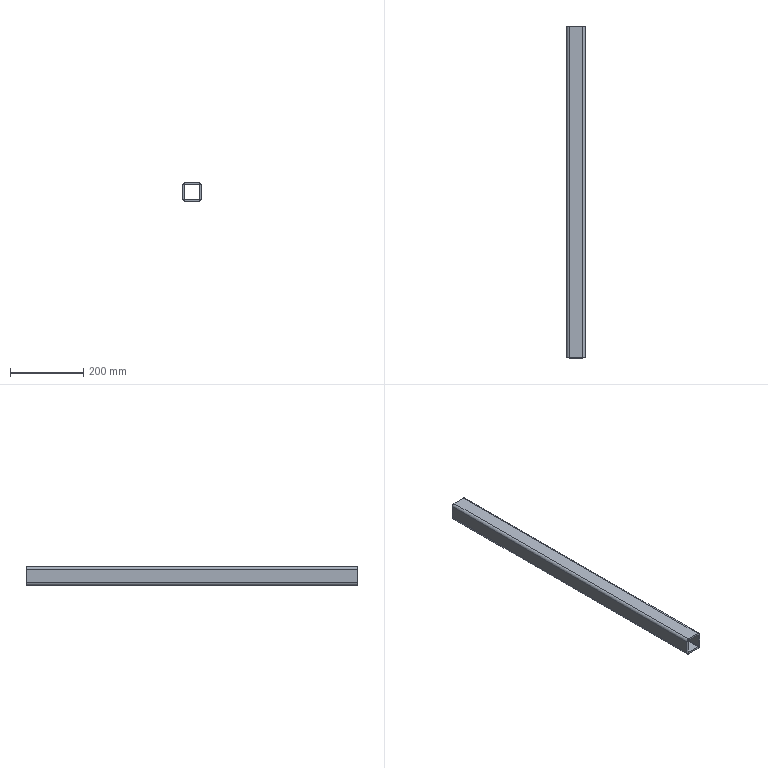Part | NX | 1 solid | 21 faces | box 50 x 906 x 50 mm | volume 780195 mm3 | cylinder 11 | plane 10 | commonest cylinder face diameters 4 x4 14 x4 4.2 x3
STEP:
#1=CARTESIAN_POINT('',(-957.,-25.,600.));
#2=VERTEX_POINT('',#1);
#3=CARTESIAN_POINT('',(-957.,881.,600.));
#4=VERTEX_POINT('',#3);
#5=CARTESIAN_POINT('',(-957.,0.,600.));
#6=DIRECTION('',(0.,1.,0.));
#7=VECTOR('',#6,1000.);
#8=LINE('',#5,#7);
#9=EDGE_CURVE('',#2,#4,#8,.T.);
#10=ORIENTED_EDGE('',*,*,#9,.F.);
#11=CARTESIAN_POINT('',(-950.,-25.,593.));
#12=VERTEX_POINT('',#11);
#13=CARTESIAN_POINT('',(-957.,-25.,593.));
#14=DIRECTION('',(0.,-1.,0.));
#15=DIRECTION('',(1.,0.,0.));
#16=AXIS2_PLACEMENT_3D('',#13,#14,#15);
#17=CIRCLE('',#16,7.);
#18=EDGE_CURVE('',#12,#2,#17,.T.);
#19=ORIENTED_EDGE('',*,*,#18,.F.);
#20=CARTESIAN_POINT('',(-950.,881.,593.));
#21=VERTEX_POINT('',#20);
#22=CARTESIAN_POINT('',(-950.,0.,593.));
#23=DIRECTION('',(0.,1.,0.));
#24=VECTOR('',#23,1000.);
#25=LINE('',#22,#24);
#26=EDGE_CURVE('',#12,#21,#25,.T.);
#27=ORIENTED_EDGE('',*,*,#26,.T.);
#28=CARTESIAN_POINT('',(-957.,881.,593.));
#29=DIRECTION('',(0.,1.,0.));
#30=DIRECTION('',(-1.,0.,0.));
#31=AXIS2_PLACEMENT_3D('',#28,#29,#30);
#32=CIRCLE('',#31,7.);
#33=EDGE_CURVE('',#4,#21,#32,.T.);
#34=ORIENTED_EDGE('',*,*,#33,.F.);
#35=EDGE_LOOP('',(#10,#19,#27,#34));
#36=FACE_BOUND('',#35,.T.);
#37=CARTESIAN_POINT('',(-957.,0.,593.));
#38=DIRECTION('',(0.,1.,0.));
#39=DIRECTION('',(-1.,0.,0.));
#40=AXIS2_PLACEMENT_3D('',#37,#38,#39);
#41=CYLINDRICAL_SURFACE('',#40,7.);
#42=ADVANCED_FACE('',(#36),#41,.T.);
#43=CARTESIAN_POINT('',(-993.,-25.,600.));
#44=VERTEX_POINT('',#43);
#45=CARTESIAN_POINT('',(-993.,881.,600.));
#46=VERTEX_POINT('',#45);
#47=CARTESIAN_POINT('',(-993.,0.,600.));
#48=DIRECTION('',(0.,1.,0.));
#49=VECTOR('',#48,1000.);
#50=LINE('',#47,#49);
#51=EDGE_CURVE('',#44,#46,#50,.T.);
#52=ORIENTED_EDGE('',*,*,#51,.F.);
#53=CARTESIAN_POINT('',(-957.,-25.,600.));
#54=DIRECTION('',(-1.,0.,0.));
#55=VECTOR('',#54,1000.);
#56=LINE('',#53,#55);
#57=EDGE_CURVE('',#2,#44,#56,.T.);
#58=ORIENTED_EDGE('',*,*,#57,.F.);
#59=ORIENTED_EDGE('',*,*,#9,.T.);
#60=CARTESIAN_POINT('',(-957.,881.,600.));
#61=DIRECTION('',(1.,0.,0.));
#62=VECTOR('',#61,1000.);
#63=LINE('',#60,#62);
#64=EDGE_CURVE('',#46,#4,#63,.T.);
#65=ORIENTED_EDGE('',*,*,#64,.F.);
#66=EDGE_LOOP('',(#52,#58,#59,#65));
#67=FACE_BOUND('',#66,.T.);
#68=CARTESIAN_POINT('',(-957.,0.,600.));
#69=DIRECTION('',(0.,0.,-1.));
#70=DIRECTION('',(-1.,0.,0.));
#71=AXIS2_PLACEMENT_3D('',#68,#69,#70);
#72=PLANE('',#71);
#73=ADVANCED_FACE('',(#67),#72,.F.);
#74=CARTESIAN_POINT('',(-1000.,-25.,593.));
#75=VERTEX_POINT('',#74);
#76=CARTESIAN_POINT('',(-1000.,881.,593.));
#77=VERTEX_POINT('',#76);
#78=CARTESIAN_POINT('',(-1000.,0.,593.));
#79=DIRECTION('',(0.,1.,0.));
#80=VECTOR('',#79,1000.);
#81=LINE('',#78,#80);
#82=EDGE_CURVE('',#75,#77,#81,.T.);
#83=ORIENTED_EDGE('',*,*,#82,.F.);
#84=CARTESIAN_POINT('',(-993.,-25.,593.));
#85=DIRECTION('',(0.,-1.,0.));
#86=DIRECTION('',(1.,0.,0.));
#87=AXIS2_PLACEMENT_3D('',#84,#85,#86);
#88=CIRCLE('',#87,7.);
#89=EDGE_CURVE('',#44,#75,#88,.T.);
#90=ORIENTED_EDGE('',*,*,#89,.F.);
#91=ORIENTED_EDGE('',*,*,#51,.T.);
#92=CARTESIAN_POINT('',(-993.,881.,593.));
#93=DIRECTION('',(0.,1.,0.));
#94=DIRECTION('',(-1.,0.,0.));
#95=AXIS2_PLACEMENT_3D('',#92,#93,#94);
#96=CIRCLE('',#95,7.);
#97=EDGE_CURVE('',#77,#46,#96,.T.);
#98=ORIENTED_EDGE('',*,*,#97,.F.);
#99=EDGE_LOOP('',(#83,#90,#91,#98));
#100=FACE_BOUND('',#99,.T.);
#101=CARTESIAN_POINT('',(-993.,0.,593.));
#102=DIRECTION('',(0.,1.,0.));
#103=DIRECTION('',(-1.,0.,0.));
#104=AXIS2_PLACEMENT_3D('',#101,#102,#103);
#105=CYLINDRICAL_SURFACE('',#104,7.);
#106=ADVANCED_FACE('',(#100),#105,.T.);
#107=CARTESIAN_POINT('',(-1000.,-25.,557.));
#108=VERTEX_POINT('',#107);
#109=CARTESIAN_POINT('',(-1000.,881.,557.));
#110=VERTEX_POINT('',#109);
#111=CARTESIAN_POINT('',(-1000.,0.,557.));
#112=DIRECTION('',(0.,1.,0.));
#113=VECTOR('',#112,1000.);
#114=LINE('',#111,#113);
#115=EDGE_CURVE('',#108,#110,#114,.T.);
#116=ORIENTED_EDGE('',*,*,#115,.F.);
#117=CARTESIAN_POINT('',(-1000.,-25.,557.));
#118=DIRECTION('',(0.,0.,-1.));
#119=VECTOR('',#118,1000.);
#120=LINE('',#117,#119);
#121=EDGE_CURVE('',#75,#108,#120,.T.);
#122=ORIENTED_EDGE('',*,*,#121,.F.);
#123=ORIENTED_EDGE('',*,*,#82,.T.);
#124=CARTESIAN_POINT('',(-1000.,881.,557.));
#125=DIRECTION('',(0.,0.,1.));
#126=VECTOR('',#125,1000.);
#127=LINE('',#124,#126);
#128=EDGE_CURVE('',#110,#77,#127,.T.);
#129=ORIENTED_EDGE('',*,*,#128,.F.);
#130=EDGE_LOOP('',(#116,#122,#123,#129));
#131=FACE_BOUND('',#130,.T.);
#132=CARTESIAN_POINT('',(-1000.,0.,557.));
#133=DIRECTION('',(1.,0.,0.));
#134=DIRECTION('',(0.,1.,0.));
#135=AXIS2_PLACEMENT_3D('',#132,#133,#134);
#136=PLANE('',#135);
#137=ADVANCED_FACE('',(#131),#136,.F.);
#138=CARTESIAN_POINT('',(-993.,-25.,550.));
#139=VERTEX_POINT('',#138);
#140=CARTESIAN_POINT('',(-993.,881.,550.));
#141=VERTEX_POINT('',#140);
#142=CARTESIAN_POINT('',(-993.,0.,550.));
#143=DIRECTION('',(0.,1.,0.));
#144=VECTOR('',#143,1000.);
#145=LINE('',#142,#144);
#146=EDGE_CURVE('',#139,#141,#145,.T.);
#147=ORIENTED_EDGE('',*,*,#146,.F.);
#148=CARTESIAN_POINT('',(-993.,-25.,557.));
#149=DIRECTION('',(0.,-1.,0.));
#150=DIRECTION('',(1.,0.,0.));
#151=AXIS2_PLACEMENT_3D('',#148,#149,#150);
#152=CIRCLE('',#151,7.);
#153=EDGE_CURVE('',#108,#139,#152,.T.);
#154=ORIENTED_EDGE('',*,*,#153,.F.);
#155=ORIENTED_EDGE('',*,*,#115,.T.);
#156=CARTESIAN_POINT('',(-993.,881.,557.));
#157=DIRECTION('',(0.,1.,0.));
#158=DIRECTION('',(-1.,0.,0.));
#159=AXIS2_PLACEMENT_3D('',#156,#157,#158);
#160=CIRCLE('',#159,7.);
#161=EDGE_CURVE('',#141,#110,#160,.T.);
#162=ORIENTED_EDGE('',*,*,#161,.F.);
#163=EDGE_LOOP('',(#147,#154,#155,#162));
#164=FACE_BOUND('',#163,.T.);
#165=CARTESIAN_POINT('',(-993.,0.,557.));
#166=DIRECTION('',(0.,1.,0.));
#167=DIRECTION('',(-1.,0.,0.));
#168=AXIS2_PLACEMENT_3D('',#165,#166,#167);
#169=CYLINDRICAL_SURFACE('',#168,7.);
#170=ADVANCED_FACE('',(#164),#169,.T.);
#171=CARTESIAN_POINT('',(-975.,133.1,550.));
#172=VERTEX_POINT('',#171);
#173=CARTESIAN_POINT('',(-975.,131.,550.));
#174=DIRECTION('',(0.,0.,-1.));
#175=DIRECTION('',(0.,1.,0.));
#176=AXIS2_PLACEMENT_3D('',#173,#174,#175);
#177=CIRCLE('',#176,2.1);
#178=EDGE_CURVE('',#172,#172,#177,.T.);
#179=ORIENTED_EDGE('',*,*,#178,.F.);
#180=EDGE_LOOP('',(#179));
#181=FACE_BOUND('',#180,.T.);
#182=CARTESIAN_POINT('',(-975.,433.1,550.));
#183=VERTEX_POINT('',#182);
#184=CARTESIAN_POINT('',(-975.,431.,550.));
#185=DIRECTION('',(0.,0.,-1.));
#186=DIRECTION('',(0.,1.,0.));
#187=AXIS2_PLACEMENT_3D('',#184,#185,#186);
#188=CIRCLE('',#187,2.1);
#189=EDGE_CURVE('',#183,#183,#188,.T.);
#190=ORIENTED_EDGE('',*,*,#189,.F.);
#191=EDGE_LOOP('',(#190));
#192=FACE_BOUND('',#191,.T.);
#193=CARTESIAN_POINT('',(-975.,733.1,550.));
#194=VERTEX_POINT('',#193);
#195=CARTESIAN_POINT('',(-975.,731.,550.));
#196=DIRECTION('',(0.,0.,-1.));
#197=DIRECTION('',(0.,1.,0.));
#198=AXIS2_PLACEMENT_3D('',#195,#196,#197);
#199=CIRCLE('',#198,2.1);
#200=EDGE_CURVE('',#194,#194,#199,.T.);
#201=ORIENTED_EDGE('',*,*,#200,.F.);
#202=EDGE_LOOP('',(#201));
#203=FACE_BOUND('',#202,.T.);
#204=CARTESIAN_POINT('',(-957.,-25.,550.));
#205=VERTEX_POINT('',#204);
#206=CARTESIAN_POINT('',(-957.,881.,550.));
#207=VERTEX_POINT('',#206);
#208=CARTESIAN_POINT('',(-957.,0.,550.));
#209=DIRECTION('',(0.,1.,0.));
#210=VECTOR('',#209,1000.);
#211=LINE('',#208,#210);
#212=EDGE_CURVE('',#205,#207,#211,.T.);
#213=ORIENTED_EDGE('',*,*,#212,.F.);
#214=CARTESIAN_POINT('',(-993.,-25.,550.));
#215=DIRECTION('',(1.,0.,0.));
#216=VECTOR('',#215,1000.);
#217=LINE('',#214,#216);
#218=EDGE_CURVE('',#139,#205,#217,.T.);
#219=ORIENTED_EDGE('',*,*,#218,.F.);
#220=ORIENTED_EDGE('',*,*,#146,.T.);
#221=CARTESIAN_POINT('',(-993.,881.,550.));
#222=DIRECTION('',(-1.,0.,0.));
#223=VECTOR('',#222,1000.);
#224=LINE('',#221,#223);
#225=EDGE_CURVE('',#207,#141,#224,.T.);
#226=ORIENTED_EDGE('',*,*,#225,.F.);
#227=EDGE_LOOP('',(#213,#219,#220,#226));
#228=FACE_BOUND('',#227,.T.);
#229=CARTESIAN_POINT('',(-993.,0.,550.));
#230=DIRECTION('',(0.,0.,1.));
#231=DIRECTION('',(1.,0.,0.));
#232=AXIS2_PLACEMENT_3D('',#229,#230,#231);
#233=PLANE('',#232);
#234=ADVANCED_FACE('',(#181,#192,#203,#228),#233,.F.);
#235=CARTESIAN_POINT('',(-950.,-25.,557.));
#236=VERTEX_POINT('',#235);
#237=CARTESIAN_POINT('',(-950.,881.,557.));
#238=VERTEX_POINT('',#237);
#239=CARTESIAN_POINT('',(-950.,0.,557.));
#240=DIRECTION('',(0.,1.,0.));
#241=VECTOR('',#240,1000.);
#242=LINE('',#239,#241);
#243=EDGE_CURVE('',#236,#238,#242,.T.);
#244=ORIENTED_EDGE('',*,*,#243,.F.);
#245=CARTESIAN_POINT('',(-957.,-25.,557.));
#246=DIRECTION('',(0.,-1.,0.));
#247=DIRECTION('',(1.,0.,0.));
#248=AXIS2_PLACEMENT_3D('',#245,#246,#247);
#249=CIRCLE('',#248,7.);
#250=EDGE_CURVE('',#205,#236,#249,.T.);
#251=ORIENTED_EDGE('',*,*,#250,.F.);
#252=ORIENTED_EDGE('',*,*,#212,.T.);
#253=CARTESIAN_POINT('',(-957.,881.,557.));
#254=DIRECTION('',(0.,1.,0.));
#255=DIRECTION('',(-1.,0.,0.));
#256=AXIS2_PLACEMENT_3D('',#253,#254,#255);
#257=CIRCLE('',#256,7.);
#258=EDGE_CURVE('',#238,#207,#257,.T.);
#259=ORIENTED_EDGE('',*,*,#258,.F.);
#260=EDGE_LOOP('',(#244,#251,#252,#259));
#261=FACE_BOUND('',#260,.T.);
#262=CARTESIAN_POINT('',(-957.,0.,557.));
#263=DIRECTION('',(0.,1.,0.));
#264=DIRECTION('',(-1.,0.,0.));
#265=AXIS2_PLACEMENT_3D('',#262,#263,#264);
#266=CYLINDRICAL_SURFACE('',#265,7.);
#267=ADVANCED_FACE('',(#261),#266,.T.);
#268=CARTESIAN_POINT('',(-993.,-25.,595.));
#269=VERTEX_POINT('',#268);
#270=CARTESIAN_POINT('',(-993.,881.,595.));
#271=VERTEX_POINT('',#270);
#272=CARTESIAN_POINT('',(-993.,0.,595.));
#273=DIRECTION('',(0.,1.,0.));
#274=VECTOR('',#273,1000.);
#275=LINE('',#272,#274);
#276=EDGE_CURVE('',#269,#271,#275,.T.);
#277=ORIENTED_EDGE('',*,*,#276,.F.);
#278=CARTESIAN_POINT('',(-995.,-25.,593.));
#279=VERTEX_POINT('',#278);
#280=CARTESIAN_POINT('',(-993.,-25.,593.));
#281=DIRECTION('',(0.,-1.,0.));
#282=DIRECTION('',(1.,0.,0.));
#283=AXIS2_PLACEMENT_3D('',#280,#281,#282);
#284=CIRCLE('',#283,2.);
#285=EDGE_CURVE('',#269,#279,#284,.T.);
#286=ORIENTED_EDGE('',*,*,#285,.T.);
#287=CARTESIAN_POINT('',(-995.,881.,593.));
#288=VERTEX_POINT('',#287);
#289=CARTESIAN_POINT('',(-995.,0.,593.));
#290=DIRECTION('',(0.,1.,0.));
#291=VECTOR('',#290,1000.);
#292=LINE('',#289,#291);
#293=EDGE_CURVE('',#279,#288,#292,.T.);
#294=ORIENTED_EDGE('',*,*,#293,.T.);
#295=CARTESIAN_POINT('',(-993.,881.,593.));
#296=DIRECTION('',(0.,1.,0.));
#297=DIRECTION('',(-1.,0.,0.));
#298=AXIS2_PLACEMENT_3D('',#295,#296,#297);
#299=CIRCLE('',#298,2.);
#300=EDGE_CURVE('',#288,#271,#299,.T.);
#301=ORIENTED_EDGE('',*,*,#300,.T.);
#302=EDGE_LOOP('',(#277,#286,#294,#301));
#303=FACE_BOUND('',#302,.T.);
#304=CARTESIAN_POINT('',(-993.,0.,593.));
#305=DIRECTION('',(0.,1.,0.));
#306=DIRECTION('',(-1.,0.,0.));
#307=AXIS2_PLACEMENT_3D('',#304,#305,#306);
#308=CYLINDRICAL_SURFACE('',#307,2.);
#309=ADVANCED_FACE('',(#303),#308,.F.);
#310=CARTESIAN_POINT('',(-957.,-25.,595.));
#311=VERTEX_POINT('',#310);
#312=CARTESIAN_POINT('',(-957.,881.,595.));
#313=VERTEX_POINT('',#312);
#314=CARTESIAN_POINT('',(-957.,0.,595.));
#315=DIRECTION('',(0.,1.,0.));
#316=VECTOR('',#315,1000.);
#317=LINE('',#314,#316);
#318=EDGE_CURVE('',#311,#313,#317,.T.);
#319=ORIENTED_EDGE('',*,*,#318,.F.);
#320=CARTESIAN_POINT('',(-957.,-25.,595.));
#321=DIRECTION('',(-1.,0.,0.));
#322=VECTOR('',#321,1000.);
#323=LINE('',#320,#322);
#324=EDGE_CURVE('',#311,#269,#323,.T.);
#325=ORIENTED_EDGE('',*,*,#324,.T.);
#326=ORIENTED_EDGE('',*,*,#276,.T.);
#327=CARTESIAN_POINT('',(-957.,881.,595.));
#328=DIRECTION('',(1.,0.,0.));
#329=VECTOR('',#328,1000.);
#330=LINE('',#327,#329);
#331=EDGE_CURVE('',#271,#313,#330,.T.);
#332=ORIENTED_EDGE('',*,*,#331,.T.);
#333=EDGE_LOOP('',(#319,#325,#326,#332));
#334=FACE_BOUND('',#333,.T.);
#335=CARTESIAN_POINT('',(-957.,0.,595.));
#336=DIRECTION('',(0.,0.,-1.));
#337=DIRECTION('',(-1.,0.,0.));
#338=AXIS2_PLACEMENT_3D('',#335,#336,#337);
#339=PLANE('',#338);
#340=ADVANCED_FACE('',(#334),#339,.T.);
#341=CARTESIAN_POINT('',(-955.,-25.,593.));
#342=VERTEX_POINT('',#341);
#343=CARTESIAN_POINT('',(-955.,881.,593.));
#344=VERTEX_POINT('',#343);
#345=CARTESIAN_POINT('',(-955.,0.,593.));
#346=DIRECTION('',(0.,1.,0.));
#347=VECTOR('',#346,1000.);
#348=LINE('',#345,#347);
#349=EDGE_CURVE('',#342,#344,#348,.T.);
#350=ORIENTED_EDGE('',*,*,#349,.F.);
#351=CARTESIAN_POINT('',(-957.,-25.,593.));
#352=DIRECTION('',(0.,-1.,0.));
#353=DIRECTION('',(1.,0.,0.));
#354=AXIS2_PLACEMENT_3D('',#351,#352,#353);
#355=CIRCLE('',#354,2.);
#356=EDGE_CURVE('',#342,#311,#355,.T.);
#357=ORIENTED_EDGE('',*,*,#356,.T.);
#358=ORIENTED_EDGE('',*,*,#318,.T.);
#359=CARTESIAN_POINT('',(-957.,881.,593.));
#360=DIRECTION('',(0.,1.,0.));
#361=DIRECTION('',(-1.,0.,0.));
#362=AXIS2_PLACEMENT_3D('',#359,#360,#361);
#363=CIRCLE('',#362,2.);
#364=EDGE_CURVE('',#313,#344,#363,.T.);
#365=ORIENTED_EDGE('',*,*,#364,.T.);
#366=EDGE_LOOP('',(#350,#357,#358,#365));
#367=FACE_BOUND('',#366,.T.);
#368=CARTESIAN_POINT('',(-957.,0.,593.));
#369=DIRECTION('',(0.,1.,0.));
#370=DIRECTION('',(-1.,0.,0.));
#371=AXIS2_PLACEMENT_3D('',#368,#369,#370);
#372=CYLINDRICAL_SURFACE('',#371,2.);
#373=ADVANCED_FACE('',(#367),#372,.F.);
#374=CARTESIAN_POINT('',(-955.,-25.,557.));
#375=VERTEX_POINT('',#374);
#376=CARTESIAN_POINT('',(-955.,881.,557.));
#377=VERTEX_POINT('',#376);
#378=CARTESIAN_POINT('',(-955.,0.,557.));
#379=DIRECTION('',(0.,1.,0.));
#380=VECTOR('',#379,1000.);
#381=LINE('',#378,#380);
#382=EDGE_CURVE('',#375,#377,#381,.T.);
#383=ORIENTED_EDGE('',*,*,#382,.F.);
#384=CARTESIAN_POINT('',(-955.,-25.,593.));
#385=DIRECTION('',(0.,0.,1.));
#386=VECTOR('',#385,1000.);
#387=LINE('',#384,#386);
#388=EDGE_CURVE('',#375,#342,#387,.T.);
#389=ORIENTED_EDGE('',*,*,#388,.T.);
#390=ORIENTED_EDGE('',*,*,#349,.T.);
#391=CARTESIAN_POINT('',(-955.,881.,593.));
#392=DIRECTION('',(0.,0.,-1.));
#393=VECTOR('',#392,1000.);
#394=LINE('',#391,#393);
#395=EDGE_CURVE('',#344,#377,#394,.T.);
#396=ORIENTED_EDGE('',*,*,#395,.T.);
#397=EDGE_LOOP('',(#383,#389,#390,#396));
#398=FACE_BOUND('',#397,.T.);
#399=CARTESIAN_POINT('',(-955.,0.,593.));
#400=DIRECTION('',(-1.,0.,0.));
#401=DIRECTION('',(0.,-1.,0.));
#402=AXIS2_PLACEMENT_3D('',#399,#400,#401);
#403=PLANE('',#402);
#404=ADVANCED_FACE('',(#398),#403,.T.);
#405=CARTESIAN_POINT('',(-957.,-25.,555.));
#406=VERTEX_POINT('',#405);
#407=CARTESIAN_POINT('',(-957.,881.,555.));
#408=VERTEX_POINT('',#407);
#409=CARTESIAN_POINT('',(-957.,0.,555.));
#410=DIRECTION('',(0.,1.,0.));
#411=VECTOR('',#410,1000.);
#412=LINE('',#409,#411);
#413=EDGE_CURVE('',#406,#408,#412,.T.);
#414=ORIENTED_EDGE('',*,*,#413,.F.);
#415=CARTESIAN_POINT('',(-957.,-25.,557.));
#416=DIRECTION('',(0.,-1.,0.));
#417=DIRECTION('',(1.,0.,0.));
#418=AXIS2_PLACEMENT_3D('',#415,#416,#417);
#419=CIRCLE('',#418,2.);
#420=EDGE_CURVE('',#406,#375,#419,.T.);
#421=ORIENTED_EDGE('',*,*,#420,.T.);
#422=ORIENTED_EDGE('',*,*,#382,.T.);
#423=CARTESIAN_POINT('',(-957.,881.,557.));
#424=DIRECTION('',(0.,1.,0.));
#425=DIRECTION('',(-1.,0.,0.));
#426=AXIS2_PLACEMENT_3D('',#423,#424,#425);
#427=CIRCLE('',#426,2.);
#428=EDGE_CURVE('',#377,#408,#427,.T.);
#429=ORIENTED_EDGE('',*,*,#428,.T.);
#430=EDGE_LOOP('',(#414,#421,#422,#429));
#431=FACE_BOUND('',#430,.T.);
#432=CARTESIAN_POINT('',(-957.,0.,557.));
#433=DIRECTION('',(0.,1.,0.));
#434=DIRECTION('',(-1.,0.,0.));
#435=AXIS2_PLACEMENT_3D('',#432,#433,#434);
#436=CYLINDRICAL_SURFACE('',#435,2.);
#437=ADVANCED_FACE('',(#431),#436,.F.);
#438=CARTESIAN_POINT('',(-972.9,131.,555.));
#439=VERTEX_POINT('',#438);
#440=CARTESIAN_POINT('',(-975.,131.,555.));
#441=DIRECTION('',(0.,0.,1.));
#442=DIRECTION('',(1.,0.,0.));
#443=AXIS2_PLACEMENT_3D('',#440,#441,#442);
#444=CIRCLE('',#443,2.1);
#445=EDGE_CURVE('',#439,#439,#444,.T.);
#446=ORIENTED_EDGE('',*,*,#445,.F.);
#447=EDGE_LOOP('',(#446));
#448=FACE_BOUND('',#447,.T.);
#449=CARTESIAN_POINT('',(-972.9,431.,555.));
#450=VERTEX_POINT('',#449);
#451=CARTESIAN_POINT('',(-975.,431.,555.));
#452=DIRECTION('',(0.,0.,1.));
#453=DIRECTION('',(1.,0.,0.));
#454=AXIS2_PLACEMENT_3D('',#451,#452,#453);
#455=CIRCLE('',#454,2.1);
#456=EDGE_CURVE('',#450,#450,#455,.T.);
#457=ORIENTED_EDGE('',*,*,#456,.F.);
#458=EDGE_LOOP('',(#457));
#459=FACE_BOUND('',#458,.T.);
#460=CARTESIAN_POINT('',(-972.9,731.,555.));
#461=VERTEX_POINT('',#460);
#462=CARTESIAN_POINT('',(-975.,731.,555.));
#463=DIRECTION('',(0.,0.,1.));
#464=DIRECTION('',(1.,0.,0.));
#465=AXIS2_PLACEMENT_3D('',#462,#463,#464);
#466=CIRCLE('',#465,2.1);
#467=EDGE_CURVE('',#461,#461,#466,.T.);
#468=ORIENTED_EDGE('',*,*,#467,.F.);
#469=EDGE_LOOP('',(#468));
#470=FACE_BOUND('',#469,.T.);
#471=CARTESIAN_POINT('',(-993.,-25.,555.));
#472=VERTEX_POINT('',#471);
#473=CARTESIAN_POINT('',(-993.,881.,555.));
#474=VERTEX_POINT('',#473);
#475=CARTESIAN_POINT('',(-993.,0.,555.));
#476=DIRECTION('',(0.,1.,0.));
#477=VECTOR('',#476,1000.);
#478=LINE('',#475,#477);
#479=EDGE_CURVE('',#472,#474,#478,.T.);
#480=ORIENTED_EDGE('',*,*,#479,.F.);
#481=CARTESIAN_POINT('',(-993.,-25.,555.));
#482=DIRECTION('',(1.,0.,0.));
#483=VECTOR('',#482,1000.);
#484=LINE('',#481,#483);
#485=EDGE_CURVE('',#472,#406,#484,.T.);
#486=ORIENTED_EDGE('',*,*,#485,.T.);
#487=ORIENTED_EDGE('',*,*,#413,.T.);
#488=CARTESIAN_POINT('',(-993.,881.,555.));
#489=DIRECTION('',(-1.,0.,0.));
#490=VECTOR('',#489,1000.);
#491=LINE('',#488,#490);
#492=EDGE_CURVE('',#408,#474,#491,.T.);
#493=ORIENTED_EDGE('',*,*,#492,.T.);
#494=EDGE_LOOP('',(#480,#486,#487,#493));
#495=FACE_BOUND('',#494,.T.);
#496=CARTESIAN_POINT('',(-993.,0.,555.));
#497=DIRECTION('',(0.,0.,1.));
#498=DIRECTION('',(1.,0.,0.));
#499=AXIS2_PLACEMENT_3D('',#496,#497,#498);
#500=PLANE('',#499);
#501=ADVANCED_FACE('',(#448,#459,#470,#495),#500,.T.);
#502=CARTESIAN_POINT('',(-995.,-25.,557.));
#503=VERTEX_POINT('',#502);
#504=CARTESIAN_POINT('',(-995.,881.,557.));
#505=VERTEX_POINT('',#504);
#506=CARTESIAN_POINT('',(-995.,0.,557.));
#507=DIRECTION('',(0.,1.,0.));
#508=VECTOR('',#507,1000.);
#509=LINE('',#506,#508);
#510=EDGE_CURVE('',#503,#505,#509,.T.);
#511=ORIENTED_EDGE('',*,*,#510,.F.);
#512=CARTESIAN_POINT('',(-993.,-25.,557.));
#513=DIRECTION('',(0.,-1.,0.));
#514=DIRECTION('',(1.,0.,0.));
#515=AXIS2_PLACEMENT_3D('',#512,#513,#514);
#516=CIRCLE('',#515,2.);
#517=EDGE_CURVE('',#503,#472,#516,.T.);
#518=ORIENTED_EDGE('',*,*,#517,.T.);
#519=ORIENTED_EDGE('',*,*,#479,.T.);
#520=CARTESIAN_POINT('',(-993.,881.,557.));
#521=DIRECTION('',(0.,1.,0.));
#522=DIRECTION('',(-1.,0.,0.));
#523=AXIS2_PLACEMENT_3D('',#520,#521,#522);
#524=CIRCLE('',#523,2.);
#525=EDGE_CURVE('',#474,#505,#524,.T.);
#526=ORIENTED_EDGE('',*,*,#525,.T.);
#527=EDGE_LOOP('',(#511,#518,#519,#526));
#528=FACE_BOUND('',#527,.T.);
#529=CARTESIAN_POINT('',(-993.,0.,557.));
#530=DIRECTION('',(0.,1.,0.));
#531=DIRECTION('',(-1.,0.,0.));
#532=AXIS2_PLACEMENT_3D('',#529,#530,#531);
#533=CYLINDRICAL_SURFACE('',#532,2.);
#534=ADVANCED_FACE('',(#528),#533,.F.);
#535=ORIENTED_EDGE('',*,*,#293,.F.);
#536=CARTESIAN_POINT('',(-995.,-25.,557.));
#537=DIRECTION('',(0.,0.,-1.));
#538=VECTOR('',#537,1000.);
#539=LINE('',#536,#538);
#540=EDGE_CURVE('',#279,#503,#539,.T.);
#541=ORIENTED_EDGE('',*,*,#540,.T.);
#542=ORIENTED_EDGE('',*,*,#510,.T.);
#543=CARTESIAN_POINT('',(-995.,881.,557.));
#544=DIRECTION('',(0.,0.,1.));
#545=VECTOR('',#544,1000.);
#546=LINE('',#543,#545);
#547=EDGE_CURVE('',#505,#288,#546,.T.);
#548=ORIENTED_EDGE('',*,*,#547,.T.);
#549=EDGE_LOOP('',(#535,#541,#542,#548));
#550=FACE_BOUND('',#549,.T.);
#551=CARTESIAN_POINT('',(-995.,0.,557.));
#552=DIRECTION('',(1.,0.,0.));
#553=DIRECTION('',(0.,1.,0.));
#554=AXIS2_PLACEMENT_3D('',#551,#552,#553);
#555=PLANE('',#554);
#556=ADVANCED_FACE('',(#550),#555,.T.);
#557=ORIENTED_EDGE('',*,*,#26,.F.);
#558=CARTESIAN_POINT('',(-950.,-25.,593.));
#559=DIRECTION('',(0.,0.,1.));
#560=VECTOR('',#559,1000.);
#561=LINE('',#558,#560);
#562=EDGE_CURVE('',#236,#12,#561,.T.);
#563=ORIENTED_EDGE('',*,*,#562,.F.);
#564=ORIENTED_EDGE('',*,*,#243,.T.);
#565=CARTESIAN_POINT('',(-950.,881.,593.));
#566=DIRECTION('',(0.,0.,-1.));
#567=VECTOR('',#566,1000.);
#568=LINE('',#565,#567);
#569=EDGE_CURVE('',#21,#238,#568,.T.);
#570=ORIENTED_EDGE('',*,*,#569,.F.);
#571=EDGE_LOOP('',(#557,#563,#564,#570));
#572=FACE_BOUND('',#571,.T.);
#573=CARTESIAN_POINT('',(-950.,0.,593.));
#574=DIRECTION('',(-1.,0.,0.));
#575=DIRECTION('',(0.,-1.,0.));
#576=AXIS2_PLACEMENT_3D('',#573,#574,#575);
#577=PLANE('',#576);
#578=ADVANCED_FACE('',(#572),#577,.F.);
#579=ORIENTED_EDGE('',*,*,#300,.F.);
#580=ORIENTED_EDGE('',*,*,#547,.F.);
#581=ORIENTED_EDGE('',*,*,#525,.F.);
#582=ORIENTED_EDGE('',*,*,#492,.F.);
#583=ORIENTED_EDGE('',*,*,#428,.F.);
#584=ORIENTED_EDGE('',*,*,#395,.F.);
#585=ORIENTED_EDGE('',*,*,#364,.F.);
#586=ORIENTED_EDGE('',*,*,#331,.F.);
#587=EDGE_LOOP('',(#579,#580,#581,#582,#583,#584,#585,#586));
#588=FACE_BOUND('',#587,.T.);
#589=ORIENTED_EDGE('',*,*,#64,.T.);
#590=ORIENTED_EDGE('',*,*,#33,.T.);
#591=ORIENTED_EDGE('',*,*,#569,.T.);
#592=ORIENTED_EDGE('',*,*,#258,.T.);
#593=ORIENTED_EDGE('',*,*,#225,.T.);
#594=ORIENTED_EDGE('',*,*,#161,.T.);
#595=ORIENTED_EDGE('',*,*,#128,.T.);
#596=ORIENTED_EDGE('',*,*,#97,.T.);
#597=EDGE_LOOP('',(#589,#590,#591,#592,#593,#594,#595,#596));
#598=FACE_BOUND('',#597,.T.);
#599=CARTESIAN_POINT('',(975.,881.,0.));
#600=DIRECTION('',(0.,1.,0.));
#601=DIRECTION('',(-1.,0.,0.));
#602=AXIS2_PLACEMENT_3D('',#599,#600,#601);
#603=PLANE('',#602);
#604=ADVANCED_FACE('',(#588,#598),#603,.T.);
#605=ORIENTED_EDGE('',*,*,#285,.F.);
#606=ORIENTED_EDGE('',*,*,#324,.F.);
#607=ORIENTED_EDGE('',*,*,#356,.F.);
#608=ORIENTED_EDGE('',*,*,#388,.F.);
#609=ORIENTED_EDGE('',*,*,#420,.F.);
#610=ORIENTED_EDGE('',*,*,#485,.F.);
#611=ORIENTED_EDGE('',*,*,#517,.F.);
#612=ORIENTED_EDGE('',*,*,#540,.F.);
#613=EDGE_LOOP('',(#605,#606,#607,#608,#609,#610,#611,#612));
#614=FACE_BOUND('',#613,.T.);
#615=ORIENTED_EDGE('',*,*,#562,.T.);
#616=ORIENTED_EDGE('',*,*,#18,.T.);
#617=ORIENTED_EDGE('',*,*,#57,.T.);
#618=ORIENTED_EDGE('',*,*,#89,.T.);
#619=ORIENTED_EDGE('',*,*,#121,.T.);
#620=ORIENTED_EDGE('',*,*,#153,.T.);
#621=ORIENTED_EDGE('',*,*,#218,.T.);
#622=ORIENTED_EDGE('',*,*,#250,.T.);
#623=EDGE_LOOP('',(#615,#616,#617,#618,#619,#620,#621,#622));
#624=FACE_BOUND('',#623,.T.);
#625=CARTESIAN_POINT('',(975.,-25.,0.));
#626=DIRECTION('',(0.,-1.,0.));
#627=DIRECTION('',(1.,0.,0.));
#628=AXIS2_PLACEMENT_3D('',#625,#626,#627);
#629=PLANE('',#628);
#630=ADVANCED_FACE('',(#614,#624),#629,.T.);
#631=ORIENTED_EDGE('',*,*,#467,.T.);
#632=EDGE_LOOP('',(#631));
#633=FACE_BOUND('',#632,.T.);
#634=ORIENTED_EDGE('',*,*,#200,.T.);
#635=EDGE_LOOP('',(#634));
#636=FACE_BOUND('',#635,.T.);
#637=CARTESIAN_POINT('',(-975.,731.,550.));
#638=DIRECTION('',(0.,0.,-1.));
#639=DIRECTION('',(0.,1.,0.));
#640=AXIS2_PLACEMENT_3D('',#637,#638,#639);
#641=CYLINDRICAL_SURFACE('',#640,2.1);
#642=ADVANCED_FACE('',(#633,#636),#641,.F.);
#643=ORIENTED_EDGE('',*,*,#456,.T.);
#644=EDGE_LOOP('',(#643));
#645=FACE_BOUND('',#644,.T.);
#646=ORIENTED_EDGE('',*,*,#189,.T.);
#647=EDGE_LOOP('',(#646));
#648=FACE_BOUND('',#647,.T.);
#649=CARTESIAN_POINT('',(-975.,431.,550.));
#650=DIRECTION('',(0.,0.,-1.));
#651=DIRECTION('',(0.,1.,0.));
#652=AXIS2_PLACEMENT_3D('',#649,#650,#651);
#653=CYLINDRICAL_SURFACE('',#652,2.1);
#654=ADVANCED_FACE('',(#645,#648),#653,.F.);
#655=ORIENTED_EDGE('',*,*,#445,.T.);
#656=EDGE_LOOP('',(#655));
#657=FACE_BOUND('',#656,.T.);
#658=ORIENTED_EDGE('',*,*,#178,.T.);
#659=EDGE_LOOP('',(#658));
#660=FACE_BOUND('',#659,.T.);
#661=CARTESIAN_POINT('',(-975.,131.,550.));
#662=DIRECTION('',(0.,0.,-1.));
#663=DIRECTION('',(0.,1.,0.));
#664=AXIS2_PLACEMENT_3D('',#661,#662,#663);
#665=CYLINDRICAL_SURFACE('',#664,2.1);
#666=ADVANCED_FACE('',(#657,#660),#665,.F.);
#667=CLOSED_SHELL('',(#42,#73,#106,#137,#170,#234,#267,#309,#340,#373,#404,#437,#501,#534,#556,#578,#604,#630,#642,#654,#666));
#668=MANIFOLD_SOLID_BREP('',#667);
#669=(LENGTH_UNIT()NAMED_UNIT(*)SI_UNIT(.MILLI.,.METRE.));
#670=UNCERTAINTY_MEASURE_WITH_UNIT(LENGTH_MEASURE(0.00001),#669,'','');
#671=(NAMED_UNIT(*)PLANE_ANGLE_UNIT()SI_UNIT($,.RADIAN.));
#672=(NAMED_UNIT(*)SI_UNIT($,.STERADIAN.)SOLID_ANGLE_UNIT());
#673=(GEOMETRIC_REPRESENTATION_CONTEXT(3)GLOBAL_UNCERTAINTY_ASSIGNED_CONTEXT((#670))GLOBAL_UNIT_ASSIGNED_CONTEXT((#669,#671,#672))REPRESENTATION_CONTEXT('',''));
#674=ADVANCED_BREP_SHAPE_REPRESENTATION('',(#668),#673);